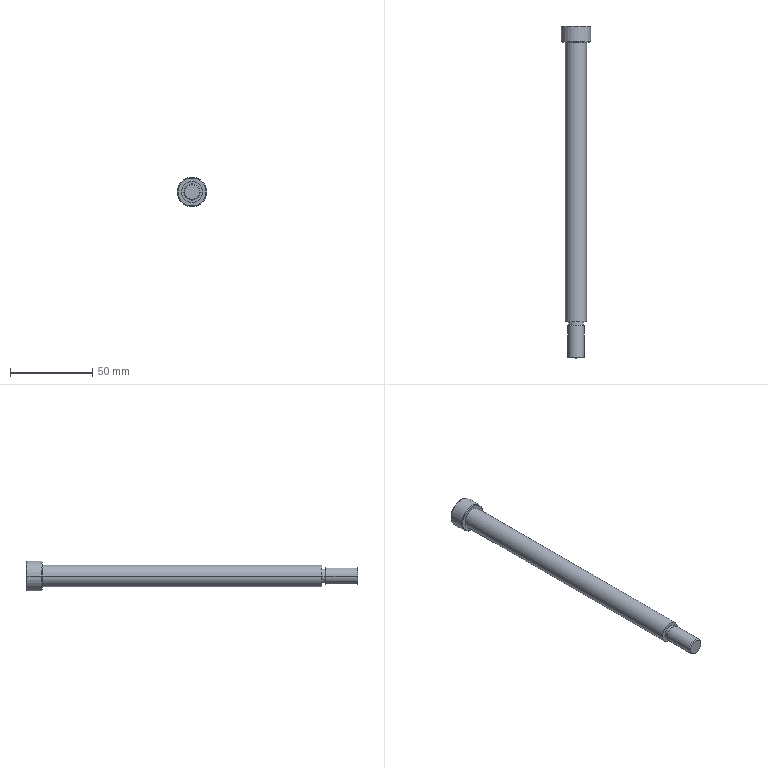Part | Creo | 1 solid | 27 faces | box 18 x 202 x 18 mm | volume 26564 mm3 | plane 11 | cone 8 | cylinder 8 | commonest cylinder face diameters 9 x2 10 x2 13 x2 18 x2
STEP:
#1=CARTESIAN_POINT('',(0.,0.,0.));
#2=DIRECTION('',(0.,0.,1.));
#3=DIRECTION('',(1.,0.,0.));
#4=AXIS2_PLACEMENT_3D('',#1,#2,#3);
#5=CARTESIAN_POINT('',(-8.55,385.,-11.133));
#6=VERTEX_POINT('',#5);
#7=CARTESIAN_POINT('',(8.45,385.,-11.133));
#8=VERTEX_POINT('',#7);
#9=CARTESIAN_POINT('',(-0.05,385.,-11.133));
#10=DIRECTION('',(0.,1.,0.));
#11=DIRECTION('',(-1.,0.,0.));
#12=AXIS2_PLACEMENT_3D('',#9,#10,#11);
#13=CIRCLE('',#12,8.5);
#14=EDGE_CURVE('',#6,#8,#13,.T.);
#15=ORIENTED_EDGE('',*,*,#14,.F.);
#16=CARTESIAN_POINT('',(-0.05,385.,-11.133));
#17=DIRECTION('',(0.,1.,0.));
#18=DIRECTION('',(1.,0.,0.));
#19=AXIS2_PLACEMENT_3D('',#16,#17,#18);
#20=CIRCLE('',#19,8.5);
#21=EDGE_CURVE('',#8,#6,#20,.T.);
#22=ORIENTED_EDGE('',*,*,#21,.F.);
#23=EDGE_LOOP('',(#15,#22));
#24=FACE_OUTER_BOUND('',#23,.F.);
#25=CARTESIAN_POINT('',(-4.669,385.,-11.133));
#26=VERTEX_POINT('',#25);
#27=CARTESIAN_POINT('',(-2.359,385.,-15.133));
#28=VERTEX_POINT('',#27);
#29=CARTESIAN_POINT('',(-4.669,385.,-11.133));
#30=DIRECTION('',(0.5,0.,-0.866));
#31=VECTOR('',#30,4.619);
#32=LINE('',#29,#31);
#33=EDGE_CURVE('',#26,#28,#32,.T.);
#34=ORIENTED_EDGE('',*,*,#33,.F.);
#35=CARTESIAN_POINT('',(-2.359,385.,-7.133));
#36=VERTEX_POINT('',#35);
#37=CARTESIAN_POINT('',(-2.359,385.,-7.133));
#38=DIRECTION('',(-0.5,0.,-0.866));
#39=VECTOR('',#38,4.619);
#40=LINE('',#37,#39);
#41=EDGE_CURVE('',#36,#26,#40,.T.);
#42=ORIENTED_EDGE('',*,*,#41,.F.);
#43=CARTESIAN_POINT('',(2.259,385.,-7.133));
#44=VERTEX_POINT('',#43);
#45=CARTESIAN_POINT('',(2.259,385.,-7.133));
#46=DIRECTION('',(-1.,0.,0.));
#47=VECTOR('',#46,4.619);
#48=LINE('',#45,#47);
#49=EDGE_CURVE('',#44,#36,#48,.T.);
#50=ORIENTED_EDGE('',*,*,#49,.F.);
#51=CARTESIAN_POINT('',(4.569,385.,-11.133));
#52=VERTEX_POINT('',#51);
#53=CARTESIAN_POINT('',(4.569,385.,-11.133));
#54=DIRECTION('',(-0.5,0.,0.866));
#55=VECTOR('',#54,4.619);
#56=LINE('',#53,#55);
#57=EDGE_CURVE('',#52,#44,#56,.T.);
#58=ORIENTED_EDGE('',*,*,#57,.F.);
#59=CARTESIAN_POINT('',(2.259,385.,-15.133));
#60=VERTEX_POINT('',#59);
#61=CARTESIAN_POINT('',(2.259,385.,-15.133));
#62=DIRECTION('',(0.5,0.,0.866));
#63=VECTOR('',#62,4.619);
#64=LINE('',#61,#63);
#65=EDGE_CURVE('',#60,#52,#64,.T.);
#66=ORIENTED_EDGE('',*,*,#65,.F.);
#67=CARTESIAN_POINT('',(-2.359,385.,-15.133));
#68=DIRECTION('',(1.,0.,0.));
#69=VECTOR('',#68,4.619);
#70=LINE('',#67,#69);
#71=EDGE_CURVE('',#28,#60,#70,.T.);
#72=ORIENTED_EDGE('',*,*,#71,.F.);
#73=EDGE_LOOP('',(#34,#42,#50,#58,#66,#72));
#74=FACE_BOUND('',#73,.F.);
#75=CARTESIAN_POINT('',(-0.05,385.,-11.133));
#76=DIRECTION('',(0.,1.,0.));
#77=DIRECTION('',(-1.,0.,0.));
#78=AXIS2_PLACEMENT_3D('',#75,#76,#77);
#79=PLANE('',#78);
#80=ADVANCED_FACE('',(#24,#74),#79,.T.);
#81=ORIENTED_EDGE('',*,*,#33,.T.);
#82=CARTESIAN_POINT('',(-2.359,381.,-15.133));
#83=VERTEX_POINT('',#82);
#84=CARTESIAN_POINT('',(-2.359,381.,-15.133));
#85=DIRECTION('',(0.,1.,0.));
#86=VECTOR('',#85,4.);
#87=LINE('',#84,#86);
#88=EDGE_CURVE('',#83,#28,#87,.T.);
#89=ORIENTED_EDGE('',*,*,#88,.F.);
#90=CARTESIAN_POINT('',(-4.669,381.,-11.133));
#91=VERTEX_POINT('',#90);
#92=CARTESIAN_POINT('',(-2.359,381.,-15.133));
#93=DIRECTION('',(-0.5,0.,0.866));
#94=VECTOR('',#93,4.619);
#95=LINE('',#92,#94);
#96=EDGE_CURVE('',#83,#91,#95,.T.);
#97=ORIENTED_EDGE('',*,*,#96,.T.);
#98=CARTESIAN_POINT('',(-4.669,381.,-11.133));
#99=DIRECTION('',(0.,1.,0.));
#100=VECTOR('',#99,4.);
#101=LINE('',#98,#100);
#102=EDGE_CURVE('',#91,#26,#101,.T.);
#103=ORIENTED_EDGE('',*,*,#102,.T.);
#104=EDGE_LOOP('',(#81,#89,#97,#103));
#105=FACE_OUTER_BOUND('',#104,.F.);
#106=CARTESIAN_POINT('',(-2.359,381.,-15.133));
#107=DIRECTION('',(-0.866,0.,-0.5));
#108=DIRECTION('',(0.5,0.,-0.866));
#109=AXIS2_PLACEMENT_3D('',#106,#107,#108);
#110=PLANE('',#109);
#111=ADVANCED_FACE('',(#105),#110,.F.);
#112=ORIENTED_EDGE('',*,*,#71,.T.);
#113=CARTESIAN_POINT('',(2.259,381.,-15.133));
#114=VERTEX_POINT('',#113);
#115=CARTESIAN_POINT('',(2.259,381.,-15.133));
#116=DIRECTION('',(0.,1.,0.));
#117=VECTOR('',#116,4.);
#118=LINE('',#115,#117);
#119=EDGE_CURVE('',#114,#60,#118,.T.);
#120=ORIENTED_EDGE('',*,*,#119,.F.);
#121=CARTESIAN_POINT('',(2.259,381.,-15.133));
#122=DIRECTION('',(-1.,0.,0.));
#123=VECTOR('',#122,4.619);
#124=LINE('',#121,#123);
#125=EDGE_CURVE('',#114,#83,#124,.T.);
#126=ORIENTED_EDGE('',*,*,#125,.T.);
#127=ORIENTED_EDGE('',*,*,#88,.T.);
#128=EDGE_LOOP('',(#112,#120,#126,#127));
#129=FACE_OUTER_BOUND('',#128,.F.);
#130=CARTESIAN_POINT('',(2.259,381.,-15.133));
#131=DIRECTION('',(0.,0.,-1.));
#132=DIRECTION('',(1.,0.,0.));
#133=AXIS2_PLACEMENT_3D('',#130,#131,#132);
#134=PLANE('',#133);
#135=ADVANCED_FACE('',(#129),#134,.F.);
#136=ORIENTED_EDGE('',*,*,#65,.T.);
#137=CARTESIAN_POINT('',(4.569,381.,-11.133));
#138=VERTEX_POINT('',#137);
#139=CARTESIAN_POINT('',(4.569,381.,-11.133));
#140=DIRECTION('',(0.,1.,0.));
#141=VECTOR('',#140,4.);
#142=LINE('',#139,#141);
#143=EDGE_CURVE('',#138,#52,#142,.T.);
#144=ORIENTED_EDGE('',*,*,#143,.F.);
#145=CARTESIAN_POINT('',(4.569,381.,-11.133));
#146=DIRECTION('',(-0.5,0.,-0.866));
#147=VECTOR('',#146,4.619);
#148=LINE('',#145,#147);
#149=EDGE_CURVE('',#138,#114,#148,.T.);
#150=ORIENTED_EDGE('',*,*,#149,.T.);
#151=ORIENTED_EDGE('',*,*,#119,.T.);
#152=EDGE_LOOP('',(#136,#144,#150,#151));
#153=FACE_OUTER_BOUND('',#152,.F.);
#154=CARTESIAN_POINT('',(4.569,381.,-11.133));
#155=DIRECTION('',(0.866,0.,-0.5));
#156=DIRECTION('',(0.5,0.,0.866));
#157=AXIS2_PLACEMENT_3D('',#154,#155,#156);
#158=PLANE('',#157);
#159=ADVANCED_FACE('',(#153),#158,.F.);
#160=ORIENTED_EDGE('',*,*,#57,.T.);
#161=CARTESIAN_POINT('',(2.259,381.,-7.133));
#162=VERTEX_POINT('',#161);
#163=CARTESIAN_POINT('',(2.259,381.,-7.133));
#164=DIRECTION('',(0.,1.,0.));
#165=VECTOR('',#164,4.);
#166=LINE('',#163,#165);
#167=EDGE_CURVE('',#162,#44,#166,.T.);
#168=ORIENTED_EDGE('',*,*,#167,.F.);
#169=CARTESIAN_POINT('',(2.259,381.,-7.133));
#170=DIRECTION('',(0.5,0.,-0.866));
#171=VECTOR('',#170,4.619);
#172=LINE('',#169,#171);
#173=EDGE_CURVE('',#162,#138,#172,.T.);
#174=ORIENTED_EDGE('',*,*,#173,.T.);
#175=ORIENTED_EDGE('',*,*,#143,.T.);
#176=EDGE_LOOP('',(#160,#168,#174,#175));
#177=FACE_OUTER_BOUND('',#176,.F.);
#178=CARTESIAN_POINT('',(2.259,381.,-7.133));
#179=DIRECTION('',(0.866,0.,0.5));
#180=DIRECTION('',(-0.5,0.,0.866));
#181=AXIS2_PLACEMENT_3D('',#178,#179,#180);
#182=PLANE('',#181);
#183=ADVANCED_FACE('',(#177),#182,.F.);
#184=ORIENTED_EDGE('',*,*,#49,.T.);
#185=CARTESIAN_POINT('',(-2.359,381.,-7.133));
#186=VERTEX_POINT('',#185);
#187=CARTESIAN_POINT('',(-2.359,381.,-7.133));
#188=DIRECTION('',(0.,1.,0.));
#189=VECTOR('',#188,4.);
#190=LINE('',#187,#189);
#191=EDGE_CURVE('',#186,#36,#190,.T.);
#192=ORIENTED_EDGE('',*,*,#191,.F.);
#193=CARTESIAN_POINT('',(-2.359,381.,-7.133));
#194=DIRECTION('',(1.,0.,0.));
#195=VECTOR('',#194,4.619);
#196=LINE('',#193,#195);
#197=EDGE_CURVE('',#186,#162,#196,.T.);
#198=ORIENTED_EDGE('',*,*,#197,.T.);
#199=ORIENTED_EDGE('',*,*,#167,.T.);
#200=EDGE_LOOP('',(#184,#192,#198,#199));
#201=FACE_OUTER_BOUND('',#200,.F.);
#202=CARTESIAN_POINT('',(-2.359,381.,-7.133));
#203=DIRECTION('',(0.,0.,1.));
#204=DIRECTION('',(-1.,0.,0.));
#205=AXIS2_PLACEMENT_3D('',#202,#203,#204);
#206=PLANE('',#205);
#207=ADVANCED_FACE('',(#201),#206,.F.);
#208=ORIENTED_EDGE('',*,*,#41,.T.);
#209=ORIENTED_EDGE('',*,*,#102,.F.);
#210=CARTESIAN_POINT('',(-4.669,381.,-11.133));
#211=DIRECTION('',(0.5,0.,0.866));
#212=VECTOR('',#211,4.619);
#213=LINE('',#210,#212);
#214=EDGE_CURVE('',#91,#186,#213,.T.);
#215=ORIENTED_EDGE('',*,*,#214,.T.);
#216=ORIENTED_EDGE('',*,*,#191,.T.);
#217=EDGE_LOOP('',(#208,#209,#215,#216));
#218=FACE_OUTER_BOUND('',#217,.F.);
#219=CARTESIAN_POINT('',(-4.669,381.,-11.133));
#220=DIRECTION('',(-0.866,0.,0.5));
#221=DIRECTION('',(-0.5,0.,-0.866));
#222=AXIS2_PLACEMENT_3D('',#219,#220,#221);
#223=PLANE('',#222);
#224=ADVANCED_FACE('',(#218),#223,.F.);
#225=ORIENTED_EDGE('',*,*,#96,.F.);
#226=ORIENTED_EDGE('',*,*,#125,.F.);
#227=ORIENTED_EDGE('',*,*,#149,.F.);
#228=ORIENTED_EDGE('',*,*,#173,.F.);
#229=ORIENTED_EDGE('',*,*,#197,.F.);
#230=ORIENTED_EDGE('',*,*,#214,.F.);
#231=EDGE_LOOP('',(#225,#226,#227,#228,#229,#230));
#232=FACE_OUTER_BOUND('',#231,.F.);
#233=CARTESIAN_POINT('',(-0.05,381.,-11.133));
#234=DIRECTION('',(0.,1.,0.));
#235=DIRECTION('',(-1.,0.,0.));
#236=AXIS2_PLACEMENT_3D('',#233,#234,#235);
#237=PLANE('',#236);
#238=ADVANCED_FACE('',(#232),#237,.T.);
#239=CARTESIAN_POINT('',(-9.05,384.5,-11.133));
#240=VERTEX_POINT('',#239);
#241=CARTESIAN_POINT('',(8.95,384.5,-11.133));
#242=VERTEX_POINT('',#241);
#243=CARTESIAN_POINT('',(-0.05,384.5,-11.133));
#244=DIRECTION('',(0.,1.,0.));
#245=DIRECTION('',(-1.,0.,0.));
#246=AXIS2_PLACEMENT_3D('',#243,#244,#245);
#247=CIRCLE('',#246,9.);
#248=EDGE_CURVE('',#240,#242,#247,.T.);
#249=ORIENTED_EDGE('',*,*,#248,.F.);
#250=CARTESIAN_POINT('',(-8.55,385.,-11.133));
#251=DIRECTION('',(-0.7071,-0.7071,0.));
#252=VECTOR('',#251,0.7071);
#253=LINE('',#250,#252);
#254=EDGE_CURVE('',#6,#240,#253,.T.);
#255=ORIENTED_EDGE('',*,*,#254,.F.);
#256=ORIENTED_EDGE('',*,*,#14,.T.);
#257=CARTESIAN_POINT('',(8.45,385.,-11.133));
#258=DIRECTION('',(0.7071,-0.7071,0.));
#259=VECTOR('',#258,0.7071);
#260=LINE('',#257,#259);
#261=EDGE_CURVE('',#8,#242,#260,.T.);
#262=ORIENTED_EDGE('',*,*,#261,.T.);
#263=EDGE_LOOP('',(#249,#255,#256,#262));
#264=FACE_OUTER_BOUND('',#263,.F.);
#265=CARTESIAN_POINT('',(-0.05,384.75,-11.133));
#266=DIRECTION('',(0.,-1.,0.));
#267=DIRECTION('',(1.,0.,0.));
#268=AXIS2_PLACEMENT_3D('',#265,#266,#267);
#269=CONICAL_SURFACE('',#268,8.75,45.);
#270=ADVANCED_FACE('',(#264),#269,.T.);
#271=CARTESIAN_POINT('',(8.95,375.5,-11.133));
#272=VERTEX_POINT('',#271);
#273=CARTESIAN_POINT('',(-9.05,375.5,-11.133));
#274=VERTEX_POINT('',#273);
#275=CARTESIAN_POINT('',(-0.05,375.5,-11.133));
#276=DIRECTION('',(0.,-1.,0.));
#277=DIRECTION('',(1.,0.,0.));
#278=AXIS2_PLACEMENT_3D('',#275,#276,#277);
#279=CIRCLE('',#278,9.);
#280=EDGE_CURVE('',#272,#274,#279,.T.);
#281=ORIENTED_EDGE('',*,*,#280,.T.);
#282=CARTESIAN_POINT('',(-9.05,375.5,-11.133));
#283=DIRECTION('',(0.,1.,0.));
#284=VECTOR('',#283,9.);
#285=LINE('',#282,#284);
#286=EDGE_CURVE('',#274,#240,#285,.T.);
#287=ORIENTED_EDGE('',*,*,#286,.T.);
#288=ORIENTED_EDGE('',*,*,#248,.T.);
#289=CARTESIAN_POINT('',(8.95,375.5,-11.133));
#290=DIRECTION('',(0.,1.,0.));
#291=VECTOR('',#290,9.);
#292=LINE('',#289,#291);
#293=EDGE_CURVE('',#272,#242,#292,.T.);
#294=ORIENTED_EDGE('',*,*,#293,.F.);
#295=EDGE_LOOP('',(#281,#287,#288,#294));
#296=FACE_OUTER_BOUND('',#295,.F.);
#297=CARTESIAN_POINT('',(-0.05,205.,-11.133));
#298=DIRECTION('',(0.,1.,0.));
#299=DIRECTION('',(-1.,0.,0.));
#300=AXIS2_PLACEMENT_3D('',#297,#298,#299);
#301=CYLINDRICAL_SURFACE('',#300,9.);
#302=ADVANCED_FACE('',(#296),#301,.T.);
#303=CARTESIAN_POINT('',(8.45,375.,-11.133));
#304=VERTEX_POINT('',#303);
#305=CARTESIAN_POINT('',(-8.55,375.,-11.133));
#306=VERTEX_POINT('',#305);
#307=CARTESIAN_POINT('',(-0.05,375.,-11.133));
#308=DIRECTION('',(0.,-1.,0.));
#309=DIRECTION('',(1.,0.,0.));
#310=AXIS2_PLACEMENT_3D('',#307,#308,#309);
#311=CIRCLE('',#310,8.5);
#312=EDGE_CURVE('',#304,#306,#311,.T.);
#313=ORIENTED_EDGE('',*,*,#312,.T.);
#314=CARTESIAN_POINT('',(-8.55,375.,-11.133));
#315=DIRECTION('',(-0.7071,0.7071,0.));
#316=VECTOR('',#315,0.7071);
#317=LINE('',#314,#316);
#318=EDGE_CURVE('',#306,#274,#317,.T.);
#319=ORIENTED_EDGE('',*,*,#318,.T.);
#320=ORIENTED_EDGE('',*,*,#280,.F.);
#321=CARTESIAN_POINT('',(8.45,375.,-11.133));
#322=DIRECTION('',(0.7071,0.7071,0.));
#323=VECTOR('',#322,0.7071);
#324=LINE('',#321,#323);
#325=EDGE_CURVE('',#304,#272,#324,.T.);
#326=ORIENTED_EDGE('',*,*,#325,.F.);
#327=EDGE_LOOP('',(#313,#319,#320,#326));
#328=FACE_OUTER_BOUND('',#327,.F.);
#329=CARTESIAN_POINT('',(-0.05,375.25,-11.133));
#330=DIRECTION('',(0.,1.,0.));
#331=DIRECTION('',(-1.,0.,0.));
#332=AXIS2_PLACEMENT_3D('',#329,#330,#331);
#333=CONICAL_SURFACE('',#332,8.75,45.);
#334=ADVANCED_FACE('',(#328),#333,.T.);
#335=ORIENTED_EDGE('',*,*,#312,.F.);
#336=CARTESIAN_POINT('',(-0.05,375.,-11.133));
#337=DIRECTION('',(0.,-1.,0.));
#338=DIRECTION('',(-1.,0.,0.));
#339=AXIS2_PLACEMENT_3D('',#336,#337,#338);
#340=CIRCLE('',#339,8.5);
#341=EDGE_CURVE('',#306,#304,#340,.T.);
#342=ORIENTED_EDGE('',*,*,#341,.F.);
#343=EDGE_LOOP('',(#335,#342));
#344=FACE_OUTER_BOUND('',#343,.F.);
#345=CARTESIAN_POINT('',(-6.55,375.,-11.133));
#346=VERTEX_POINT('',#345);
#347=CARTESIAN_POINT('',(6.45,375.,-11.133));
#348=VERTEX_POINT('',#347);
#349=CARTESIAN_POINT('',(-0.05,375.,-11.133));
#350=DIRECTION('',(0.,1.,0.));
#351=DIRECTION('',(-1.,0.,0.));
#352=AXIS2_PLACEMENT_3D('',#349,#350,#351);
#353=CIRCLE('',#352,6.5);
#354=EDGE_CURVE('',#346,#348,#353,.T.);
#355=ORIENTED_EDGE('',*,*,#354,.F.);
#356=CARTESIAN_POINT('',(-0.05,375.,-11.133));
#357=DIRECTION('',(0.,1.,0.));
#358=DIRECTION('',(1.,0.,0.));
#359=AXIS2_PLACEMENT_3D('',#356,#357,#358);
#360=CIRCLE('',#359,6.5);
#361=EDGE_CURVE('',#348,#346,#360,.T.);
#362=ORIENTED_EDGE('',*,*,#361,.F.);
#363=EDGE_LOOP('',(#355,#362));
#364=FACE_BOUND('',#363,.F.);
#365=CARTESIAN_POINT('',(-0.05,375.,-2.134));
#366=DIRECTION('',(0.,-1.,0.));
#367=DIRECTION('',(1.,0.,0.));
#368=AXIS2_PLACEMENT_3D('',#365,#366,#367);
#369=PLANE('',#368);
#370=ADVANCED_FACE('',(#344,#364),#369,.T.);
#371=ORIENTED_EDGE('',*,*,#341,.T.);
#372=ORIENTED_EDGE('',*,*,#325,.T.);
#373=CARTESIAN_POINT('',(-0.05,375.5,-11.133));
#374=DIRECTION('',(0.,-1.,0.));
#375=DIRECTION('',(-1.,0.,0.));
#376=AXIS2_PLACEMENT_3D('',#373,#374,#375);
#377=CIRCLE('',#376,9.);
#378=EDGE_CURVE('',#274,#272,#377,.T.);
#379=ORIENTED_EDGE('',*,*,#378,.F.);
#380=ORIENTED_EDGE('',*,*,#318,.F.);
#381=EDGE_LOOP('',(#371,#372,#379,#380));
#382=FACE_OUTER_BOUND('',#381,.F.);
#383=CARTESIAN_POINT('',(-0.05,375.25,-11.133));
#384=DIRECTION('',(0.,1.,0.));
#385=DIRECTION('',(-1.,0.,0.));
#386=AXIS2_PLACEMENT_3D('',#383,#384,#385);
#387=CONICAL_SURFACE('',#386,8.75,45.);
#388=ADVANCED_FACE('',(#382),#387,.T.);
#389=ORIENTED_EDGE('',*,*,#378,.T.);
#390=ORIENTED_EDGE('',*,*,#293,.T.);
#391=CARTESIAN_POINT('',(-0.05,384.5,-11.133));
#392=DIRECTION('',(0.,1.,0.));
#393=DIRECTION('',(1.,0.,0.));
#394=AXIS2_PLACEMENT_3D('',#391,#392,#393);
#395=CIRCLE('',#394,9.);
#396=EDGE_CURVE('',#242,#240,#395,.T.);
#397=ORIENTED_EDGE('',*,*,#396,.T.);
#398=ORIENTED_EDGE('',*,*,#286,.F.);
#399=EDGE_LOOP('',(#389,#390,#397,#398));
#400=FACE_OUTER_BOUND('',#399,.F.);
#401=CARTESIAN_POINT('',(-0.05,205.,-11.133));
#402=DIRECTION('',(0.,1.,0.));
#403=DIRECTION('',(-1.,0.,0.));
#404=AXIS2_PLACEMENT_3D('',#401,#402,#403);
#405=CYLINDRICAL_SURFACE('',#404,9.);
#406=ADVANCED_FACE('',(#400),#405,.T.);
#407=ORIENTED_EDGE('',*,*,#396,.F.);
#408=ORIENTED_EDGE('',*,*,#261,.F.);
#409=ORIENTED_EDGE('',*,*,#21,.T.);
#410=ORIENTED_EDGE('',*,*,#254,.T.);
#411=EDGE_LOOP('',(#407,#408,#409,#410));
#412=FACE_OUTER_BOUND('',#411,.F.);
#413=CARTESIAN_POINT('',(-0.05,384.75,-11.133));
#414=DIRECTION('',(0.,-1.,0.));
#415=DIRECTION('',(1.,0.,0.));
#416=AXIS2_PLACEMENT_3D('',#413,#414,#415);
#417=CONICAL_SURFACE('',#416,8.75,45.);
#418=ADVANCED_FACE('',(#412),#417,.T.);
#419=CARTESIAN_POINT('',(6.45,205.,-11.133));
#420=VERTEX_POINT('',#419);
#421=CARTESIAN_POINT('',(-6.55,205.,-11.133));
#422=VERTEX_POINT('',#421);
#423=CARTESIAN_POINT('',(-0.05,205.,-11.133));
#424=DIRECTION('',(0.,-1.,0.));
#425=DIRECTION('',(1.,0.,0.));
#426=AXIS2_PLACEMENT_3D('',#423,#424,#425);
#427=CIRCLE('',#426,6.5);
#428=EDGE_CURVE('',#420,#422,#427,.T.);
#429=ORIENTED_EDGE('',*,*,#428,.T.);
#430=CARTESIAN_POINT('',(-6.55,205.,-11.133));
#431=DIRECTION('',(0.,1.,0.));
#432=VECTOR('',#431,170.);
#433=LINE('',#430,#432);
#434=EDGE_CURVE('',#422,#346,#433,.T.);
#435=ORIENTED_EDGE('',*,*,#434,.T.);
#436=ORIENTED_EDGE('',*,*,#354,.T.);
#437=CARTESIAN_POINT('',(6.45,205.,-11.133));
#438=DIRECTION('',(0.,1.,0.));
#439=VECTOR('',#438,170.);
#440=LINE('',#437,#439);
#441=EDGE_CURVE('',#420,#348,#440,.T.);
#442=ORIENTED_EDGE('',*,*,#441,.F.);
#443=EDGE_LOOP('',(#429,#435,#436,#442));
#444=FACE_OUTER_BOUND('',#443,.F.);
#445=CARTESIAN_POINT('',(-0.05,205.,-11.133));
#446=DIRECTION('',(0.,1.,0.));
#447=DIRECTION('',(-1.,0.,0.));
#448=AXIS2_PLACEMENT_3D('',#445,#446,#447);
#449=CYLINDRICAL_SURFACE('',#448,6.5);
#450=ADVANCED_FACE('',(#444),#449,.T.);
#451=CARTESIAN_POINT('',(-0.05,205.,-11.133));
#452=DIRECTION('',(0.,-1.,0.));
#453=DIRECTION('',(-1.,0.,0.));
#454=AXIS2_PLACEMENT_3D('',#451,#452,#453);
#455=CIRCLE('',#454,6.5);
#456=EDGE_CURVE('',#422,#420,#455,.T.);
#457=ORIENTED_EDGE('',*,*,#456,.F.);
#458=ORIENTED_EDGE('',*,*,#428,.F.);
#459=EDGE_LOOP('',(#457,#458));
#460=FACE_OUTER_BOUND('',#459,.F.);
#461=CARTESIAN_POINT('',(-4.55,205.,-11.133));
#462=VERTEX_POINT('',#461);
#463=CARTESIAN_POINT('',(4.45,205.,-11.133));
#464=VERTEX_POINT('',#463);
#465=CARTESIAN_POINT('',(-0.05,205.,-11.133));
#466=DIRECTION('',(0.,1.,0.));
#467=DIRECTION('',(-1.,0.,0.));
#468=AXIS2_PLACEMENT_3D('',#465,#466,#467);
#469=CIRCLE('',#468,4.5);
#470=EDGE_CURVE('',#462,#464,#469,.T.);
#471=ORIENTED_EDGE('',*,*,#470,.F.);
#472=CARTESIAN_POINT('',(-0.05,205.,-11.133));
#473=DIRECTION('',(0.,1.,0.));
#474=DIRECTION('',(1.,0.,0.));
#475=AXIS2_PLACEMENT_3D('',#472,#473,#474);
#476=CIRCLE('',#475,4.5);
#477=EDGE_CURVE('',#464,#462,#476,.T.);
#478=ORIENTED_EDGE('',*,*,#477,.F.);
#479=EDGE_LOOP('',(#471,#478));
#480=FACE_BOUND('',#479,.F.);
#481=CARTESIAN_POINT('',(-0.05,205.,-4.633));
#482=DIRECTION('',(0.,-1.,0.));
#483=DIRECTION('',(1.,0.,0.));
#484=AXIS2_PLACEMENT_3D('',#481,#482,#483);
#485=PLANE('',#484);
#486=ADVANCED_FACE('',(#460,#480),#485,.T.);
#487=CARTESIAN_POINT('',(4.45,203.,-11.133));
#488=VERTEX_POINT('',#487);
#489=CARTESIAN_POINT('',(-4.55,203.,-11.133));
#490=VERTEX_POINT('',#489);
#491=CARTESIAN_POINT('',(-0.05,203.,-11.133));
#492=DIRECTION('',(0.,-1.,0.));
#493=DIRECTION('',(1.,0.,0.));
#494=AXIS2_PLACEMENT_3D('',#491,#492,#493);
#495=CIRCLE('',#494,4.5);
#496=EDGE_CURVE('',#488,#490,#495,.T.);
#497=ORIENTED_EDGE('',*,*,#496,.T.);
#498=CARTESIAN_POINT('',(-4.55,203.,-11.133));
#499=DIRECTION('',(0.,1.,0.));
#500=VECTOR('',#499,2.);
#501=LINE('',#498,#500);
#502=EDGE_CURVE('',#490,#462,#501,.T.);
#503=ORIENTED_EDGE('',*,*,#502,.T.);
#504=ORIENTED_EDGE('',*,*,#470,.T.);
#505=CARTESIAN_POINT('',(4.45,203.,-11.133));
#506=DIRECTION('',(0.,1.,0.));
#507=VECTOR('',#506,2.);
#508=LINE('',#505,#507);
#509=EDGE_CURVE('',#488,#464,#508,.T.);
#510=ORIENTED_EDGE('',*,*,#509,.F.);
#511=EDGE_LOOP('',(#497,#503,#504,#510));
#512=FACE_OUTER_BOUND('',#511,.F.);
#513=CARTESIAN_POINT('',(-0.05,205.,-11.133));
#514=DIRECTION('',(0.,1.,0.));
#515=DIRECTION('',(-1.,0.,0.));
#516=AXIS2_PLACEMENT_3D('',#513,#514,#515);
#517=CYLINDRICAL_SURFACE('',#516,4.5);
#518=ADVANCED_FACE('',(#512),#517,.T.);
#519=CARTESIAN_POINT('',(-5.05,202.5,-11.133));
#520=VERTEX_POINT('',#519);
#521=CARTESIAN_POINT('',(4.95,202.5,-11.133));
#522=VERTEX_POINT('',#521);
#523=CARTESIAN_POINT('',(-0.05,202.5,-11.133));
#524=DIRECTION('',(0.,1.,0.));
#525=DIRECTION('',(-1.,0.,0.));
#526=AXIS2_PLACEMENT_3D('',#523,#524,#525);
#527=CIRCLE('',#526,5.);
#528=EDGE_CURVE('',#520,#522,#527,.T.);
#529=ORIENTED_EDGE('',*,*,#528,.F.);
#530=CARTESIAN_POINT('',(-4.55,203.,-11.133));
#531=DIRECTION('',(-0.7071,-0.7071,0.));
#532=VECTOR('',#531,0.7071);
#533=LINE('',#530,#532);
#534=EDGE_CURVE('',#490,#520,#533,.T.);
#535=ORIENTED_EDGE('',*,*,#534,.F.);
#536=ORIENTED_EDGE('',*,*,#496,.F.);
#537=CARTESIAN_POINT('',(4.45,203.,-11.133));
#538=DIRECTION('',(0.7071,-0.7071,0.));
#539=VECTOR('',#538,0.7071);
#540=LINE('',#537,#539);
#541=EDGE_CURVE('',#488,#522,#540,.T.);
#542=ORIENTED_EDGE('',*,*,#541,.T.);
#543=EDGE_LOOP('',(#529,#535,#536,#542));
#544=FACE_OUTER_BOUND('',#543,.F.);
#545=CARTESIAN_POINT('',(-0.05,202.75,-11.133));
#546=DIRECTION('',(0.,-1.,0.));
#547=DIRECTION('',(1.,0.,0.));
#548=AXIS2_PLACEMENT_3D('',#545,#546,#547);
#549=CONICAL_SURFACE('',#548,4.75,45.);
#550=ADVANCED_FACE('',(#544),#549,.T.);
#551=ORIENTED_EDGE('',*,*,#528,.T.);
#552=CARTESIAN_POINT('',(4.95,183.5,-11.133));
#553=VERTEX_POINT('',#552);
#554=CARTESIAN_POINT('',(4.95,183.5,-11.133));
#555=DIRECTION('',(0.,1.,0.));
#556=VECTOR('',#555,19.);
#557=LINE('',#554,#556);
#558=EDGE_CURVE('',#553,#522,#557,.T.);
#559=ORIENTED_EDGE('',*,*,#558,.F.);
#560=CARTESIAN_POINT('',(-5.05,183.5,-11.133));
#561=VERTEX_POINT('',#560);
#562=CARTESIAN_POINT('',(-0.05,183.5,-11.133));
#563=DIRECTION('',(0.,-1.,0.));
#564=DIRECTION('',(1.,0.,0.));
#565=AXIS2_PLACEMENT_3D('',#562,#563,#564);
#566=CIRCLE('',#565,5.);
#567=EDGE_CURVE('',#553,#561,#566,.T.);
#568=ORIENTED_EDGE('',*,*,#567,.T.);
#569=CARTESIAN_POINT('',(-5.05,183.5,-11.133));
#570=DIRECTION('',(0.,1.,0.));
#571=VECTOR('',#570,19.);
#572=LINE('',#569,#571);
#573=EDGE_CURVE('',#561,#520,#572,.T.);
#574=ORIENTED_EDGE('',*,*,#573,.T.);
#575=EDGE_LOOP('',(#551,#559,#568,#574));
#576=FACE_OUTER_BOUND('',#575,.F.);
#577=CARTESIAN_POINT('',(-0.05,205.,-11.133));
#578=DIRECTION('',(0.,1.,0.));
#579=DIRECTION('',(-1.,0.,0.));
#580=AXIS2_PLACEMENT_3D('',#577,#578,#579);
#581=CYLINDRICAL_SURFACE('',#580,5.);
#582=ADVANCED_FACE('',(#576),#581,.T.);
#583=CARTESIAN_POINT('',(-0.05,202.5,-11.133));
#584=DIRECTION('',(0.,1.,0.));
#585=DIRECTION('',(1.,0.,0.));
#586=AXIS2_PLACEMENT_3D('',#583,#584,#585);
#587=CIRCLE('',#586,5.);
#588=EDGE_CURVE('',#522,#520,#587,.T.);
#589=ORIENTED_EDGE('',*,*,#588,.T.);
#590=ORIENTED_EDGE('',*,*,#573,.F.);
#591=CARTESIAN_POINT('',(-0.05,183.5,-11.133));
#592=DIRECTION('',(0.,-1.,0.));
#593=DIRECTION('',(-1.,0.,0.));
#594=AXIS2_PLACEMENT_3D('',#591,#592,#593);
#595=CIRCLE('',#594,5.);
#596=EDGE_CURVE('',#561,#553,#595,.T.);
#597=ORIENTED_EDGE('',*,*,#596,.T.);
#598=ORIENTED_EDGE('',*,*,#558,.T.);
#599=EDGE_LOOP('',(#589,#590,#597,#598));
#600=FACE_OUTER_BOUND('',#599,.F.);
#601=CARTESIAN_POINT('',(-0.05,205.,-11.133));
#602=DIRECTION('',(0.,1.,0.));
#603=DIRECTION('',(-1.,0.,0.));
#604=AXIS2_PLACEMENT_3D('',#601,#602,#603);
#605=CYLINDRICAL_SURFACE('',#604,5.);
#606=ADVANCED_FACE('',(#600),#605,.T.);
#607=ORIENTED_EDGE('',*,*,#588,.F.);
#608=ORIENTED_EDGE('',*,*,#541,.F.);
#609=CARTESIAN_POINT('',(-0.05,203.,-11.133));
#610=DIRECTION('',(0.,-1.,0.));
#611=DIRECTION('',(-1.,0.,0.));
#612=AXIS2_PLACEMENT_3D('',#609,#610,#611);
#613=CIRCLE('',#612,4.5);
#614=EDGE_CURVE('',#490,#488,#613,.T.);
#615=ORIENTED_EDGE('',*,*,#614,.F.);
#616=ORIENTED_EDGE('',*,*,#534,.T.);
#617=EDGE_LOOP('',(#607,#608,#615,#616));
#618=FACE_OUTER_BOUND('',#617,.F.);
#619=CARTESIAN_POINT('',(-0.05,202.75,-11.133));
#620=DIRECTION('',(0.,-1.,0.));
#621=DIRECTION('',(1.,0.,0.));
#622=AXIS2_PLACEMENT_3D('',#619,#620,#621);
#623=CONICAL_SURFACE('',#622,4.75,45.);
#624=ADVANCED_FACE('',(#618),#623,.T.);
#625=ORIENTED_EDGE('',*,*,#614,.T.);
#626=ORIENTED_EDGE('',*,*,#509,.T.);
#627=ORIENTED_EDGE('',*,*,#477,.T.);
#628=ORIENTED_EDGE('',*,*,#502,.F.);
#629=EDGE_LOOP('',(#625,#626,#627,#628));
#630=FACE_OUTER_BOUND('',#629,.F.);
#631=CARTESIAN_POINT('',(-0.05,205.,-11.133));
#632=DIRECTION('',(0.,1.,0.));
#633=DIRECTION('',(-1.,0.,0.));
#634=AXIS2_PLACEMENT_3D('',#631,#632,#633);
#635=CYLINDRICAL_SURFACE('',#634,4.5);
#636=ADVANCED_FACE('',(#630),#635,.T.);
#637=CARTESIAN_POINT('',(-4.55,183.,-11.133));
#638=VERTEX_POINT('',#637);
#639=CARTESIAN_POINT('',(4.45,183.,-11.133));
#640=VERTEX_POINT('',#639);
#641=CARTESIAN_POINT('',(-0.05,183.,-11.133));
#642=DIRECTION('',(0.,-1.,0.));
#643=DIRECTION('',(-1.,0.,0.));
#644=AXIS2_PLACEMENT_3D('',#641,#642,#643);
#645=CIRCLE('',#644,4.5);
#646=EDGE_CURVE('',#638,#640,#645,.T.);
#647=ORIENTED_EDGE('',*,*,#646,.T.);
#648=CARTESIAN_POINT('',(4.45,183.,-11.133));
#649=DIRECTION('',(0.7071,0.7071,0.));
#650=VECTOR('',#649,0.7071);
#651=LINE('',#648,#650);
#652=EDGE_CURVE('',#640,#553,#651,.T.);
#653=ORIENTED_EDGE('',*,*,#652,.T.);
#654=ORIENTED_EDGE('',*,*,#596,.F.);
#655=CARTESIAN_POINT('',(-4.55,183.,-11.133));
#656=DIRECTION('',(-0.7071,0.7071,0.));
#657=VECTOR('',#656,0.7071);
#658=LINE('',#655,#657);
#659=EDGE_CURVE('',#638,#561,#658,.T.);
#660=ORIENTED_EDGE('',*,*,#659,.F.);
#661=EDGE_LOOP('',(#647,#653,#654,#660));
#662=FACE_OUTER_BOUND('',#661,.F.);
#663=CARTESIAN_POINT('',(-0.05,183.25,-11.133));
#664=DIRECTION('',(0.,1.,0.));
#665=DIRECTION('',(-1.,0.,0.));
#666=AXIS2_PLACEMENT_3D('',#663,#664,#665);
#667=CONICAL_SURFACE('',#666,4.75,45.);
#668=ADVANCED_FACE('',(#662),#667,.T.);
#669=CARTESIAN_POINT('',(-0.05,183.,-11.133));
#670=DIRECTION('',(0.,-1.,0.));
#671=DIRECTION('',(1.,0.,0.));
#672=AXIS2_PLACEMENT_3D('',#669,#670,#671);
#673=CIRCLE('',#672,4.5);
#674=EDGE_CURVE('',#640,#638,#673,.T.);
#675=ORIENTED_EDGE('',*,*,#674,.F.);
#676=ORIENTED_EDGE('',*,*,#646,.F.);
#677=EDGE_LOOP('',(#675,#676));
#678=FACE_OUTER_BOUND('',#677,.F.);
#679=CARTESIAN_POINT('',(-0.05,183.,-6.133));
#680=DIRECTION('',(0.,-1.,0.));
#681=DIRECTION('',(1.,0.,0.));
#682=AXIS2_PLACEMENT_3D('',#679,#680,#681);
#683=PLANE('',#682);
#684=ADVANCED_FACE('',(#678),#683,.T.);
#685=ORIENTED_EDGE('',*,*,#674,.T.);
#686=ORIENTED_EDGE('',*,*,#659,.T.);
#687=ORIENTED_EDGE('',*,*,#567,.F.);
#688=ORIENTED_EDGE('',*,*,#652,.F.);
#689=EDGE_LOOP('',(#685,#686,#687,#688));
#690=FACE_OUTER_BOUND('',#689,.F.);
#691=CARTESIAN_POINT('',(-0.05,183.25,-11.133));
#692=DIRECTION('',(0.,1.,0.));
#693=DIRECTION('',(-1.,0.,0.));
#694=AXIS2_PLACEMENT_3D('',#691,#692,#693);
#695=CONICAL_SURFACE('',#694,4.75,45.);
#696=ADVANCED_FACE('',(#690),#695,.T.);
#697=ORIENTED_EDGE('',*,*,#456,.T.);
#698=ORIENTED_EDGE('',*,*,#441,.T.);
#699=ORIENTED_EDGE('',*,*,#361,.T.);
#700=ORIENTED_EDGE('',*,*,#434,.F.);
#701=EDGE_LOOP('',(#697,#698,#699,#700));
#702=FACE_OUTER_BOUND('',#701,.F.);
#703=CARTESIAN_POINT('',(-0.05,205.,-11.133));
#704=DIRECTION('',(0.,1.,0.));
#705=DIRECTION('',(-1.,0.,0.));
#706=AXIS2_PLACEMENT_3D('',#703,#704,#705);
#707=CYLINDRICAL_SURFACE('',#706,6.5);
#708=ADVANCED_FACE('',(#702),#707,.T.);
#709=CLOSED_SHELL('',(#80,#111,#135,#159,#183,#207,#224,#238,#270,#302,#334,#370,#388,#406,#418,#450,#486,#518,#550,#582,#606,#624,#636,#668,#684,#696,#708));
#710=MANIFOLD_SOLID_BREP('',#709);
#711=(LENGTH_UNIT()NAMED_UNIT(*)SI_UNIT(.MILLI.,.METRE.));
#712=UNCERTAINTY_MEASURE_WITH_UNIT(LENGTH_MEASURE(0.02036),#711,'','');
#713=(NAMED_UNIT(*)PLANE_ANGLE_UNIT()SI_UNIT($,.RADIAN.));
#714=PLANE_ANGLE_MEASURE_WITH_UNIT(PLANE_ANGLE_MEASURE(0.01745),#713);
#715=(CONVERSION_BASED_UNIT('DEGREE',#714)NAMED_UNIT(*)PLANE_ANGLE_UNIT());
#716=(NAMED_UNIT(*)SI_UNIT($,.STERADIAN.)SOLID_ANGLE_UNIT());
#717=(GEOMETRIC_REPRESENTATION_CONTEXT(3)GLOBAL_UNCERTAINTY_ASSIGNED_CONTEXT((#712))GLOBAL_UNIT_ASSIGNED_CONTEXT((#711,#715,#716))REPRESENTATION_CONTEXT('',''));
#718=ADVANCED_BREP_SHAPE_REPRESENTATION('',(#4,#710),#717);